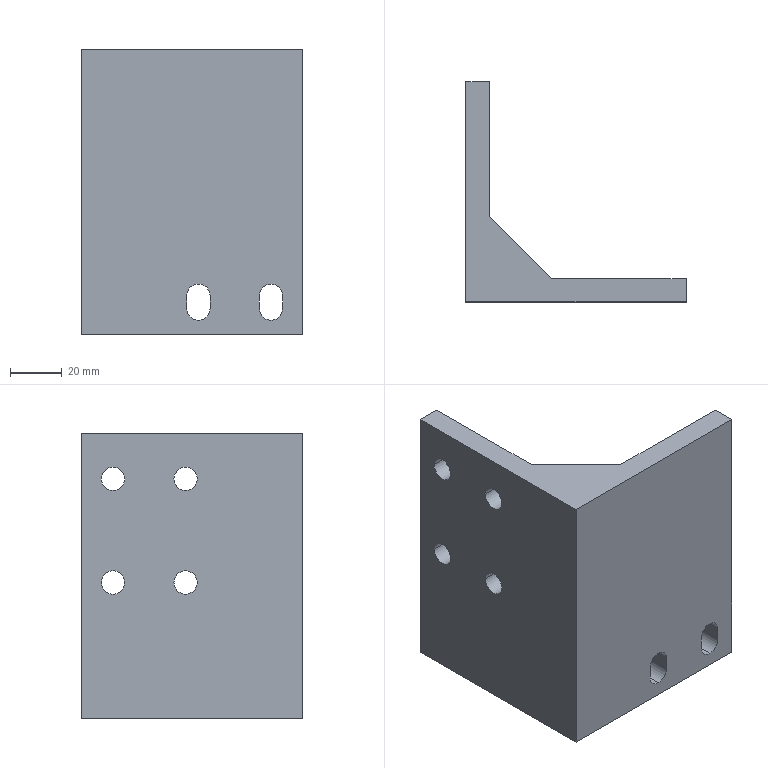Part | 1 solid | 27 faces | box 85 x 85 x 110 mm | volume 186825 mm3 | cylinder 14 | plane 13 | commonest cylinder face diameters 9 x14
STEP:
#1=CARTESIAN_POINT('',(30.5,-33.5,-67.));
#2=VERTEX_POINT('',#1);
#3=CARTESIAN_POINT('',(35.,-33.5,-62.5));
#4=VERTEX_POINT('',#3);
#5=CARTESIAN_POINT('',(30.5,-33.5,-62.5));
#6=DIRECTION('',(0.,-1.,0.));
#7=DIRECTION('',(0.,0.,-1.));
#8=AXIS2_PLACEMENT_3D('',#5,#6,#7);
#9=CIRCLE('',#8,4.5);
#10=EDGE_CURVE('',#2,#4,#9,.T.);
#11=ORIENTED_EDGE('',*,*,#10,.F.);
#12=CARTESIAN_POINT('',(30.5,-42.5,-67.));
#13=VERTEX_POINT('',#12);
#14=CARTESIAN_POINT('',(30.5,42.5,-67.));
#15=DIRECTION('',(0.,-1.,0.));
#16=VECTOR('',#15,1000.);
#17=LINE('',#14,#16);
#18=EDGE_CURVE('',#2,#13,#17,.T.);
#19=ORIENTED_EDGE('',*,*,#18,.T.);
#20=CARTESIAN_POINT('',(35.,-42.5,-62.5));
#21=VERTEX_POINT('',#20);
#22=CARTESIAN_POINT('',(30.5,-42.5,-62.5));
#23=DIRECTION('',(0.,-1.,0.));
#24=DIRECTION('',(0.,0.,-1.));
#25=AXIS2_PLACEMENT_3D('',#22,#23,#24);
#26=CIRCLE('',#25,4.5);
#27=EDGE_CURVE('',#13,#21,#26,.T.);
#28=ORIENTED_EDGE('',*,*,#27,.T.);
#29=CARTESIAN_POINT('',(35.,42.5,-62.5));
#30=DIRECTION('',(0.,-1.,0.));
#31=VECTOR('',#30,1000.);
#32=LINE('',#29,#31);
#33=EDGE_CURVE('',#4,#21,#32,.T.);
#34=ORIENTED_EDGE('',*,*,#33,.F.);
#35=EDGE_LOOP('',(#11,#19,#28,#34));
#36=FACE_OUTER_BOUND('',#35,.T.);
#37=CARTESIAN_POINT('',(30.5,42.5,-62.5));
#38=DIRECTION('',(0.,-1.,0.));
#39=DIRECTION('',(0.,0.,-1.));
#40=AXIS2_PLACEMENT_3D('',#37,#38,#39);
#41=CYLINDRICAL_SURFACE('',#40,4.5);
#42=ADVANCED_FACE('',(#36),#41,.F.);
#43=CARTESIAN_POINT('',(2.5,-33.5,-67.));
#44=VERTEX_POINT('',#43);
#45=CARTESIAN_POINT('',(7.,-33.5,-62.5));
#46=VERTEX_POINT('',#45);
#47=CARTESIAN_POINT('',(2.5,-33.5,-62.5));
#48=DIRECTION('',(0.,-1.,0.));
#49=DIRECTION('',(0.,0.,-1.));
#50=AXIS2_PLACEMENT_3D('',#47,#48,#49);
#51=CIRCLE('',#50,4.5);
#52=EDGE_CURVE('',#44,#46,#51,.T.);
#53=ORIENTED_EDGE('',*,*,#52,.F.);
#54=CARTESIAN_POINT('',(2.5,-42.5,-67.));
#55=VERTEX_POINT('',#54);
#56=CARTESIAN_POINT('',(2.5,42.5,-67.));
#57=DIRECTION('',(0.,-1.,0.));
#58=VECTOR('',#57,1000.);
#59=LINE('',#56,#58);
#60=EDGE_CURVE('',#44,#55,#59,.T.);
#61=ORIENTED_EDGE('',*,*,#60,.T.);
#62=CARTESIAN_POINT('',(7.,-42.5,-62.5));
#63=VERTEX_POINT('',#62);
#64=CARTESIAN_POINT('',(2.5,-42.5,-62.5));
#65=DIRECTION('',(0.,-1.,0.));
#66=DIRECTION('',(0.,0.,-1.));
#67=AXIS2_PLACEMENT_3D('',#64,#65,#66);
#68=CIRCLE('',#67,4.5);
#69=EDGE_CURVE('',#55,#63,#68,.T.);
#70=ORIENTED_EDGE('',*,*,#69,.T.);
#71=CARTESIAN_POINT('',(7.,42.5,-62.5));
#72=DIRECTION('',(0.,-1.,0.));
#73=VECTOR('',#72,1000.);
#74=LINE('',#71,#73);
#75=EDGE_CURVE('',#46,#63,#74,.T.);
#76=ORIENTED_EDGE('',*,*,#75,.F.);
#77=EDGE_LOOP('',(#53,#61,#70,#76));
#78=FACE_OUTER_BOUND('',#77,.T.);
#79=CARTESIAN_POINT('',(2.5,42.5,-62.5));
#80=DIRECTION('',(0.,-1.,0.));
#81=DIRECTION('',(0.,0.,-1.));
#82=AXIS2_PLACEMENT_3D('',#79,#80,#81);
#83=CYLINDRICAL_SURFACE('',#82,4.5);
#84=ADVANCED_FACE('',(#78),#83,.F.);
#85=CARTESIAN_POINT('',(-42.5,-2.,-20.));
#86=VERTEX_POINT('',#85);
#87=CARTESIAN_POINT('',(-42.5,7.,-20.));
#88=VERTEX_POINT('',#87);
#89=CARTESIAN_POINT('',(-42.5,2.5,-20.));
#90=DIRECTION('',(1.,0.,0.));
#91=DIRECTION('',(0.,1.,0.));
#92=AXIS2_PLACEMENT_3D('',#89,#90,#91);
#93=CIRCLE('',#92,4.5);
#94=EDGE_CURVE('',#86,#88,#93,.T.);
#95=ORIENTED_EDGE('',*,*,#94,.F.);
#96=CARTESIAN_POINT('',(-33.5,-2.,-20.));
#97=VERTEX_POINT('',#96);
#98=CARTESIAN_POINT('',(-42.5,-2.,-20.));
#99=DIRECTION('',(1.,0.,0.));
#100=VECTOR('',#99,1000.);
#101=LINE('',#98,#100);
#102=EDGE_CURVE('',#86,#97,#101,.T.);
#103=ORIENTED_EDGE('',*,*,#102,.T.);
#104=CARTESIAN_POINT('',(-33.5,7.,-20.));
#105=VERTEX_POINT('',#104);
#106=CARTESIAN_POINT('',(-33.5,2.5,-20.));
#107=DIRECTION('',(1.,0.,0.));
#108=DIRECTION('',(0.,1.,0.));
#109=AXIS2_PLACEMENT_3D('',#106,#107,#108);
#110=CIRCLE('',#109,4.5);
#111=EDGE_CURVE('',#97,#105,#110,.T.);
#112=ORIENTED_EDGE('',*,*,#111,.T.);
#113=CARTESIAN_POINT('',(-42.5,7.,-20.));
#114=DIRECTION('',(1.,0.,0.));
#115=VECTOR('',#114,1000.);
#116=LINE('',#113,#115);
#117=EDGE_CURVE('',#88,#105,#116,.T.);
#118=ORIENTED_EDGE('',*,*,#117,.F.);
#119=EDGE_LOOP('',(#95,#103,#112,#118));
#120=FACE_OUTER_BOUND('',#119,.T.);
#121=CARTESIAN_POINT('',(-42.5,2.5,-20.));
#122=DIRECTION('',(1.,0.,0.));
#123=DIRECTION('',(0.,1.,0.));
#124=AXIS2_PLACEMENT_3D('',#121,#122,#123);
#125=CYLINDRICAL_SURFACE('',#124,4.5);
#126=ADVANCED_FACE('',(#120),#125,.F.);
#127=CARTESIAN_POINT('',(-42.5,-2.,20.));
#128=VERTEX_POINT('',#127);
#129=CARTESIAN_POINT('',(-42.5,7.,20.));
#130=VERTEX_POINT('',#129);
#131=CARTESIAN_POINT('',(-42.5,2.5,20.));
#132=DIRECTION('',(1.,0.,0.));
#133=DIRECTION('',(0.,1.,0.));
#134=AXIS2_PLACEMENT_3D('',#131,#132,#133);
#135=CIRCLE('',#134,4.5);
#136=EDGE_CURVE('',#128,#130,#135,.T.);
#137=ORIENTED_EDGE('',*,*,#136,.F.);
#138=CARTESIAN_POINT('',(-33.5,-2.,20.));
#139=VERTEX_POINT('',#138);
#140=CARTESIAN_POINT('',(-42.5,-2.,20.));
#141=DIRECTION('',(1.,0.,0.));
#142=VECTOR('',#141,1000.);
#143=LINE('',#140,#142);
#144=EDGE_CURVE('',#128,#139,#143,.T.);
#145=ORIENTED_EDGE('',*,*,#144,.T.);
#146=CARTESIAN_POINT('',(-33.5,7.,20.));
#147=VERTEX_POINT('',#146);
#148=CARTESIAN_POINT('',(-33.5,2.5,20.));
#149=DIRECTION('',(1.,0.,0.));
#150=DIRECTION('',(0.,1.,0.));
#151=AXIS2_PLACEMENT_3D('',#148,#149,#150);
#152=CIRCLE('',#151,4.5);
#153=EDGE_CURVE('',#139,#147,#152,.T.);
#154=ORIENTED_EDGE('',*,*,#153,.T.);
#155=CARTESIAN_POINT('',(-42.5,7.,20.));
#156=DIRECTION('',(1.,0.,0.));
#157=VECTOR('',#156,1000.);
#158=LINE('',#155,#157);
#159=EDGE_CURVE('',#130,#147,#158,.T.);
#160=ORIENTED_EDGE('',*,*,#159,.F.);
#161=EDGE_LOOP('',(#137,#145,#154,#160));
#162=FACE_OUTER_BOUND('',#161,.T.);
#163=CARTESIAN_POINT('',(-42.5,2.5,20.));
#164=DIRECTION('',(1.,0.,0.));
#165=DIRECTION('',(0.,1.,0.));
#166=AXIS2_PLACEMENT_3D('',#163,#164,#165);
#167=CYLINDRICAL_SURFACE('',#166,4.5);
#168=ADVANCED_FACE('',(#162),#167,.F.);
#169=CARTESIAN_POINT('',(-42.5,26.,20.));
#170=VERTEX_POINT('',#169);
#171=CARTESIAN_POINT('',(-42.5,35.,20.));
#172=VERTEX_POINT('',#171);
#173=CARTESIAN_POINT('',(-42.5,30.5,20.));
#174=DIRECTION('',(1.,0.,0.));
#175=DIRECTION('',(0.,1.,0.));
#176=AXIS2_PLACEMENT_3D('',#173,#174,#175);
#177=CIRCLE('',#176,4.5);
#178=EDGE_CURVE('',#170,#172,#177,.T.);
#179=ORIENTED_EDGE('',*,*,#178,.F.);
#180=CARTESIAN_POINT('',(-33.5,26.,20.));
#181=VERTEX_POINT('',#180);
#182=CARTESIAN_POINT('',(-42.5,26.,20.));
#183=DIRECTION('',(1.,0.,0.));
#184=VECTOR('',#183,1000.);
#185=LINE('',#182,#184);
#186=EDGE_CURVE('',#170,#181,#185,.T.);
#187=ORIENTED_EDGE('',*,*,#186,.T.);
#188=CARTESIAN_POINT('',(-33.5,35.,20.));
#189=VERTEX_POINT('',#188);
#190=CARTESIAN_POINT('',(-33.5,30.5,20.));
#191=DIRECTION('',(1.,0.,0.));
#192=DIRECTION('',(0.,1.,0.));
#193=AXIS2_PLACEMENT_3D('',#190,#191,#192);
#194=CIRCLE('',#193,4.5);
#195=EDGE_CURVE('',#181,#189,#194,.T.);
#196=ORIENTED_EDGE('',*,*,#195,.T.);
#197=CARTESIAN_POINT('',(-42.5,35.,20.));
#198=DIRECTION('',(1.,0.,0.));
#199=VECTOR('',#198,1000.);
#200=LINE('',#197,#199);
#201=EDGE_CURVE('',#172,#189,#200,.T.);
#202=ORIENTED_EDGE('',*,*,#201,.F.);
#203=EDGE_LOOP('',(#179,#187,#196,#202));
#204=FACE_OUTER_BOUND('',#203,.T.);
#205=CARTESIAN_POINT('',(-42.5,30.5,20.));
#206=DIRECTION('',(1.,0.,0.));
#207=DIRECTION('',(0.,1.,0.));
#208=AXIS2_PLACEMENT_3D('',#205,#206,#207);
#209=CYLINDRICAL_SURFACE('',#208,4.5);
#210=ADVANCED_FACE('',(#204),#209,.F.);
#211=CARTESIAN_POINT('',(-42.5,26.,-20.));
#212=VERTEX_POINT('',#211);
#213=CARTESIAN_POINT('',(-42.5,35.,-20.));
#214=VERTEX_POINT('',#213);
#215=CARTESIAN_POINT('',(-42.5,30.5,-20.));
#216=DIRECTION('',(1.,0.,0.));
#217=DIRECTION('',(0.,1.,0.));
#218=AXIS2_PLACEMENT_3D('',#215,#216,#217);
#219=CIRCLE('',#218,4.5);
#220=EDGE_CURVE('',#212,#214,#219,.T.);
#221=ORIENTED_EDGE('',*,*,#220,.F.);
#222=CARTESIAN_POINT('',(-33.5,26.,-20.));
#223=VERTEX_POINT('',#222);
#224=CARTESIAN_POINT('',(-42.5,26.,-20.));
#225=DIRECTION('',(1.,0.,0.));
#226=VECTOR('',#225,1000.);
#227=LINE('',#224,#226);
#228=EDGE_CURVE('',#212,#223,#227,.T.);
#229=ORIENTED_EDGE('',*,*,#228,.T.);
#230=CARTESIAN_POINT('',(-33.5,35.,-20.));
#231=VERTEX_POINT('',#230);
#232=CARTESIAN_POINT('',(-33.5,30.5,-20.));
#233=DIRECTION('',(1.,0.,0.));
#234=DIRECTION('',(0.,1.,0.));
#235=AXIS2_PLACEMENT_3D('',#232,#233,#234);
#236=CIRCLE('',#235,4.5);
#237=EDGE_CURVE('',#223,#231,#236,.T.);
#238=ORIENTED_EDGE('',*,*,#237,.T.);
#239=CARTESIAN_POINT('',(-42.5,35.,-20.));
#240=DIRECTION('',(1.,0.,0.));
#241=VECTOR('',#240,1000.);
#242=LINE('',#239,#241);
#243=EDGE_CURVE('',#214,#231,#242,.T.);
#244=ORIENTED_EDGE('',*,*,#243,.F.);
#245=EDGE_LOOP('',(#221,#229,#238,#244));
#246=FACE_OUTER_BOUND('',#245,.T.);
#247=CARTESIAN_POINT('',(-42.5,30.5,-20.));
#248=DIRECTION('',(1.,0.,0.));
#249=DIRECTION('',(0.,1.,0.));
#250=AXIS2_PLACEMENT_3D('',#247,#248,#249);
#251=CYLINDRICAL_SURFACE('',#250,4.5);
#252=ADVANCED_FACE('',(#246),#251,.F.);
#253=CARTESIAN_POINT('',(-33.5,42.5,37.5));
#254=VERTEX_POINT('',#253);
#255=CARTESIAN_POINT('',(-33.5,42.5,-72.5));
#256=VERTEX_POINT('',#255);
#257=CARTESIAN_POINT('',(-33.5,42.5,37.5));
#258=DIRECTION('',(0.,0.,-1.));
#259=VECTOR('',#258,1000.);
#260=LINE('',#257,#259);
#261=EDGE_CURVE('',#254,#256,#260,.T.);
#262=ORIENTED_EDGE('',*,*,#261,.T.);
#263=CARTESIAN_POINT('',(-42.5,42.5,-72.5));
#264=VERTEX_POINT('',#263);
#265=CARTESIAN_POINT('',(42.5,42.5,-72.5));
#266=DIRECTION('',(-1.,0.,0.));
#267=VECTOR('',#266,1000.);
#268=LINE('',#265,#267);
#269=EDGE_CURVE('',#256,#264,#268,.T.);
#270=ORIENTED_EDGE('',*,*,#269,.T.);
#271=CARTESIAN_POINT('',(-42.5,42.5,37.5));
#272=VERTEX_POINT('',#271);
#273=CARTESIAN_POINT('',(-42.5,42.5,-37.5));
#274=DIRECTION('',(0.,0.,1.));
#275=VECTOR('',#274,1000.);
#276=LINE('',#273,#275);
#277=EDGE_CURVE('',#264,#272,#276,.T.);
#278=ORIENTED_EDGE('',*,*,#277,.T.);
#279=CARTESIAN_POINT('',(42.5,42.5,37.5));
#280=DIRECTION('',(-1.,0.,0.));
#281=VECTOR('',#280,1000.);
#282=LINE('',#279,#281);
#283=EDGE_CURVE('',#254,#272,#282,.T.);
#284=ORIENTED_EDGE('',*,*,#283,.F.);
#285=EDGE_LOOP('',(#262,#270,#278,#284));
#286=FACE_OUTER_BOUND('',#285,.T.);
#287=CARTESIAN_POINT('',(42.5,42.5,-37.5));
#288=DIRECTION('',(0.,1.,0.));
#289=DIRECTION('',(-1.,0.,0.));
#290=AXIS2_PLACEMENT_3D('',#287,#288,#289);
#291=PLANE('',#290);
#292=ADVANCED_FACE('',(#286),#291,.T.);
#293=CARTESIAN_POINT('',(42.5,-33.5,37.5));
#294=VERTEX_POINT('',#293);
#295=CARTESIAN_POINT('',(42.5,-33.5,-72.5));
#296=VERTEX_POINT('',#295);
#297=CARTESIAN_POINT('',(42.5,-33.5,37.5));
#298=DIRECTION('',(0.,0.,-1.));
#299=VECTOR('',#298,1000.);
#300=LINE('',#297,#299);
#301=EDGE_CURVE('',#294,#296,#300,.T.);
#302=ORIENTED_EDGE('',*,*,#301,.F.);
#303=CARTESIAN_POINT('',(42.5,-42.5,37.5));
#304=VERTEX_POINT('',#303);
#305=CARTESIAN_POINT('',(42.5,-42.5,37.5));
#306=DIRECTION('',(0.,1.,0.));
#307=VECTOR('',#306,1000.);
#308=LINE('',#305,#307);
#309=EDGE_CURVE('',#304,#294,#308,.T.);
#310=ORIENTED_EDGE('',*,*,#309,.F.);
#311=CARTESIAN_POINT('',(42.5,-42.5,-72.5));
#312=VERTEX_POINT('',#311);
#313=CARTESIAN_POINT('',(42.5,-42.5,-37.5));
#314=DIRECTION('',(0.,0.,1.));
#315=VECTOR('',#314,1000.);
#316=LINE('',#313,#315);
#317=EDGE_CURVE('',#312,#304,#316,.T.);
#318=ORIENTED_EDGE('',*,*,#317,.F.);
#319=CARTESIAN_POINT('',(42.5,-42.5,-72.5));
#320=DIRECTION('',(0.,1.,0.));
#321=VECTOR('',#320,1000.);
#322=LINE('',#319,#321);
#323=EDGE_CURVE('',#312,#296,#322,.T.);
#324=ORIENTED_EDGE('',*,*,#323,.T.);
#325=EDGE_LOOP('',(#302,#310,#318,#324));
#326=FACE_OUTER_BOUND('',#325,.T.);
#327=CARTESIAN_POINT('',(42.5,-42.5,-37.5));
#328=DIRECTION('',(1.,0.,0.));
#329=DIRECTION('',(0.,0.,-1.));
#330=AXIS2_PLACEMENT_3D('',#327,#328,#329);
#331=PLANE('',#330);
#332=ADVANCED_FACE('',(#326),#331,.T.);
#333=CARTESIAN_POINT('',(26.,-42.5,-62.5));
#334=VERTEX_POINT('',#333);
#335=CARTESIAN_POINT('',(30.5,-42.5,-62.5));
#336=DIRECTION('',(0.,-1.,0.));
#337=DIRECTION('',(0.,0.,-1.));
#338=AXIS2_PLACEMENT_3D('',#335,#336,#337);
#339=CIRCLE('',#338,4.5);
#340=EDGE_CURVE('',#334,#13,#339,.T.);
#341=ORIENTED_EDGE('',*,*,#340,.F.);
#342=CARTESIAN_POINT('',(26.,-42.5,-57.5));
#343=VERTEX_POINT('',#342);
#344=CARTESIAN_POINT('',(26.,-42.5,-62.5));
#345=DIRECTION('',(0.,0.,-1.));
#346=VECTOR('',#345,1000.);
#347=LINE('',#344,#346);
#348=EDGE_CURVE('',#343,#334,#347,.T.);
#349=ORIENTED_EDGE('',*,*,#348,.F.);
#350=CARTESIAN_POINT('',(35.,-42.5,-57.5));
#351=VERTEX_POINT('',#350);
#352=CARTESIAN_POINT('',(30.5,-42.5,-57.5));
#353=DIRECTION('',(0.,-1.,0.));
#354=DIRECTION('',(0.,0.,-1.));
#355=AXIS2_PLACEMENT_3D('',#352,#353,#354);
#356=CIRCLE('',#355,4.5);
#357=EDGE_CURVE('',#351,#343,#356,.T.);
#358=ORIENTED_EDGE('',*,*,#357,.F.);
#359=CARTESIAN_POINT('',(35.,-42.5,-62.5));
#360=DIRECTION('',(0.,0.,1.));
#361=VECTOR('',#360,1000.);
#362=LINE('',#359,#361);
#363=EDGE_CURVE('',#21,#351,#362,.T.);
#364=ORIENTED_EDGE('',*,*,#363,.F.);
#365=ORIENTED_EDGE('',*,*,#27,.F.);
#366=EDGE_LOOP('',(#341,#349,#358,#364,#365));
#367=FACE_BOUND('',#366,.T.);
#368=CARTESIAN_POINT('',(-2.,-42.5,-62.5));
#369=VERTEX_POINT('',#368);
#370=CARTESIAN_POINT('',(2.5,-42.5,-62.5));
#371=DIRECTION('',(0.,-1.,0.));
#372=DIRECTION('',(0.,0.,-1.));
#373=AXIS2_PLACEMENT_3D('',#370,#371,#372);
#374=CIRCLE('',#373,4.5);
#375=EDGE_CURVE('',#369,#55,#374,.T.);
#376=ORIENTED_EDGE('',*,*,#375,.F.);
#377=CARTESIAN_POINT('',(-2.,-42.5,-57.5));
#378=VERTEX_POINT('',#377);
#379=CARTESIAN_POINT('',(-2.,-42.5,-62.5));
#380=DIRECTION('',(0.,0.,-1.));
#381=VECTOR('',#380,1000.);
#382=LINE('',#379,#381);
#383=EDGE_CURVE('',#378,#369,#382,.T.);
#384=ORIENTED_EDGE('',*,*,#383,.F.);
#385=CARTESIAN_POINT('',(7.,-42.5,-57.5));
#386=VERTEX_POINT('',#385);
#387=CARTESIAN_POINT('',(2.5,-42.5,-57.5));
#388=DIRECTION('',(0.,-1.,0.));
#389=DIRECTION('',(0.,0.,-1.));
#390=AXIS2_PLACEMENT_3D('',#387,#388,#389);
#391=CIRCLE('',#390,4.5);
#392=EDGE_CURVE('',#386,#378,#391,.T.);
#393=ORIENTED_EDGE('',*,*,#392,.F.);
#394=CARTESIAN_POINT('',(7.,-42.5,-62.5));
#395=DIRECTION('',(0.,0.,1.));
#396=VECTOR('',#395,1000.);
#397=LINE('',#394,#396);
#398=EDGE_CURVE('',#63,#386,#397,.T.);
#399=ORIENTED_EDGE('',*,*,#398,.F.);
#400=ORIENTED_EDGE('',*,*,#69,.F.);
#401=EDGE_LOOP('',(#376,#384,#393,#399,#400));
#402=FACE_BOUND('',#401,.T.);
#403=CARTESIAN_POINT('',(-42.5,-42.5,37.5));
#404=VERTEX_POINT('',#403);
#405=CARTESIAN_POINT('',(-42.5,-42.5,37.5));
#406=DIRECTION('',(1.,0.,0.));
#407=VECTOR('',#406,1000.);
#408=LINE('',#405,#407);
#409=EDGE_CURVE('',#404,#304,#408,.T.);
#410=ORIENTED_EDGE('',*,*,#409,.F.);
#411=CARTESIAN_POINT('',(-42.5,-42.5,-72.5));
#412=VERTEX_POINT('',#411);
#413=CARTESIAN_POINT('',(-42.5,-42.5,-37.5));
#414=DIRECTION('',(0.,0.,1.));
#415=VECTOR('',#414,1000.);
#416=LINE('',#413,#415);
#417=EDGE_CURVE('',#412,#404,#416,.T.);
#418=ORIENTED_EDGE('',*,*,#417,.F.);
#419=CARTESIAN_POINT('',(-42.5,-42.5,-72.5));
#420=DIRECTION('',(1.,0.,0.));
#421=VECTOR('',#420,1000.);
#422=LINE('',#419,#421);
#423=EDGE_CURVE('',#412,#312,#422,.T.);
#424=ORIENTED_EDGE('',*,*,#423,.T.);
#425=ORIENTED_EDGE('',*,*,#317,.T.);
#426=EDGE_LOOP('',(#410,#418,#424,#425));
#427=FACE_OUTER_BOUND('',#426,.T.);
#428=CARTESIAN_POINT('',(-42.5,-42.5,-37.5));
#429=DIRECTION('',(0.,-1.,0.));
#430=DIRECTION('',(0.,0.,-1.));
#431=AXIS2_PLACEMENT_3D('',#428,#429,#430);
#432=PLANE('',#431);
#433=ADVANCED_FACE('',(#367,#402,#427),#432,.T.);
#434=CARTESIAN_POINT('',(-42.5,2.5,-20.));
#435=DIRECTION('',(1.,0.,0.));
#436=DIRECTION('',(0.,1.,0.));
#437=AXIS2_PLACEMENT_3D('',#434,#435,#436);
#438=CIRCLE('',#437,4.5);
#439=EDGE_CURVE('',#88,#86,#438,.T.);
#440=ORIENTED_EDGE('',*,*,#439,.T.);
#441=ORIENTED_EDGE('',*,*,#94,.T.);
#442=EDGE_LOOP('',(#440,#441));
#443=FACE_BOUND('',#442,.T.);
#444=CARTESIAN_POINT('',(-42.5,2.5,20.));
#445=DIRECTION('',(1.,0.,0.));
#446=DIRECTION('',(0.,1.,0.));
#447=AXIS2_PLACEMENT_3D('',#444,#445,#446);
#448=CIRCLE('',#447,4.5);
#449=EDGE_CURVE('',#130,#128,#448,.T.);
#450=ORIENTED_EDGE('',*,*,#449,.T.);
#451=ORIENTED_EDGE('',*,*,#136,.T.);
#452=EDGE_LOOP('',(#450,#451));
#453=FACE_BOUND('',#452,.T.);
#454=CARTESIAN_POINT('',(-42.5,30.5,20.));
#455=DIRECTION('',(1.,0.,0.));
#456=DIRECTION('',(0.,1.,0.));
#457=AXIS2_PLACEMENT_3D('',#454,#455,#456);
#458=CIRCLE('',#457,4.5);
#459=EDGE_CURVE('',#172,#170,#458,.T.);
#460=ORIENTED_EDGE('',*,*,#459,.T.);
#461=ORIENTED_EDGE('',*,*,#178,.T.);
#462=EDGE_LOOP('',(#460,#461));
#463=FACE_BOUND('',#462,.T.);
#464=CARTESIAN_POINT('',(-42.5,30.5,-20.));
#465=DIRECTION('',(1.,0.,0.));
#466=DIRECTION('',(0.,1.,0.));
#467=AXIS2_PLACEMENT_3D('',#464,#465,#466);
#468=CIRCLE('',#467,4.5);
#469=EDGE_CURVE('',#214,#212,#468,.T.);
#470=ORIENTED_EDGE('',*,*,#469,.T.);
#471=ORIENTED_EDGE('',*,*,#220,.T.);
#472=EDGE_LOOP('',(#470,#471));
#473=FACE_BOUND('',#472,.T.);
#474=CARTESIAN_POINT('',(-42.5,42.5,37.5));
#475=DIRECTION('',(0.,-1.,0.));
#476=VECTOR('',#475,1000.);
#477=LINE('',#474,#476);
#478=EDGE_CURVE('',#272,#404,#477,.T.);
#479=ORIENTED_EDGE('',*,*,#478,.F.);
#480=ORIENTED_EDGE('',*,*,#277,.F.);
#481=CARTESIAN_POINT('',(-42.5,42.5,-72.5));
#482=DIRECTION('',(0.,-1.,0.));
#483=VECTOR('',#482,1000.);
#484=LINE('',#481,#483);
#485=EDGE_CURVE('',#264,#412,#484,.T.);
#486=ORIENTED_EDGE('',*,*,#485,.T.);
#487=ORIENTED_EDGE('',*,*,#417,.T.);
#488=EDGE_LOOP('',(#479,#480,#486,#487));
#489=FACE_OUTER_BOUND('',#488,.T.);
#490=CARTESIAN_POINT('',(-42.5,42.5,-37.5));
#491=DIRECTION('',(-1.,0.,0.));
#492=DIRECTION('',(0.,-1.,0.));
#493=AXIS2_PLACEMENT_3D('',#490,#491,#492);
#494=PLANE('',#493);
#495=ADVANCED_FACE('',(#443,#453,#463,#473,#489),#494,.T.);
#496=ORIENTED_EDGE('',*,*,#269,.F.);
#497=CARTESIAN_POINT('',(-33.5,-9.5,-72.5));
#498=VERTEX_POINT('',#497);
#499=CARTESIAN_POINT('',(-33.5,-33.5,-72.5));
#500=DIRECTION('',(0.,1.,0.));
#501=VECTOR('',#500,1000.);
#502=LINE('',#499,#501);
#503=EDGE_CURVE('',#498,#256,#502,.T.);
#504=ORIENTED_EDGE('',*,*,#503,.F.);
#505=CARTESIAN_POINT('',(-9.5,-33.5,-72.5));
#506=VERTEX_POINT('',#505);
#507=CARTESIAN_POINT('',(-21.5,-21.5,-72.5));
#508=DIRECTION('',(0.7071,-0.7071,0.));
#509=VECTOR('',#508,1000.);
#510=LINE('',#507,#509);
#511=EDGE_CURVE('',#498,#506,#510,.T.);
#512=ORIENTED_EDGE('',*,*,#511,.T.);
#513=CARTESIAN_POINT('',(42.5,-33.5,-72.5));
#514=DIRECTION('',(-1.,0.,0.));
#515=VECTOR('',#514,1000.);
#516=LINE('',#513,#515);
#517=EDGE_CURVE('',#296,#506,#516,.T.);
#518=ORIENTED_EDGE('',*,*,#517,.F.);
#519=ORIENTED_EDGE('',*,*,#323,.F.);
#520=ORIENTED_EDGE('',*,*,#423,.F.);
#521=ORIENTED_EDGE('',*,*,#485,.F.);
#522=EDGE_LOOP('',(#496,#504,#512,#518,#519,#520,#521));
#523=FACE_OUTER_BOUND('',#522,.T.);
#524=CARTESIAN_POINT('',(0.,0.,-72.5));
#525=DIRECTION('',(0.,0.,1.));
#526=DIRECTION('',(1.,0.,0.));
#527=AXIS2_PLACEMENT_3D('',#524,#525,#526);
#528=PLANE('',#527);
#529=ADVANCED_FACE('',(#523),#528,.F.);
#530=CARTESIAN_POINT('',(-9.5,-33.5,37.5));
#531=VERTEX_POINT('',#530);
#532=CARTESIAN_POINT('',(42.5,-33.5,37.5));
#533=DIRECTION('',(-1.,0.,0.));
#534=VECTOR('',#533,1000.);
#535=LINE('',#532,#534);
#536=EDGE_CURVE('',#294,#531,#535,.T.);
#537=ORIENTED_EDGE('',*,*,#536,.T.);
#538=CARTESIAN_POINT('',(-33.5,-9.5,37.5));
#539=VERTEX_POINT('',#538);
#540=CARTESIAN_POINT('',(-33.5,-9.5,37.5));
#541=DIRECTION('',(-0.7071,0.7071,0.));
#542=VECTOR('',#541,1000.);
#543=LINE('',#540,#542);
#544=EDGE_CURVE('',#531,#539,#543,.T.);
#545=ORIENTED_EDGE('',*,*,#544,.T.);
#546=CARTESIAN_POINT('',(-33.5,-33.5,37.5));
#547=DIRECTION('',(0.,1.,0.));
#548=VECTOR('',#547,1000.);
#549=LINE('',#546,#548);
#550=EDGE_CURVE('',#539,#254,#549,.T.);
#551=ORIENTED_EDGE('',*,*,#550,.T.);
#552=ORIENTED_EDGE('',*,*,#283,.T.);
#553=ORIENTED_EDGE('',*,*,#478,.T.);
#554=ORIENTED_EDGE('',*,*,#409,.T.);
#555=ORIENTED_EDGE('',*,*,#309,.T.);
#556=EDGE_LOOP('',(#537,#545,#551,#552,#553,#554,#555));
#557=FACE_OUTER_BOUND('',#556,.T.);
#558=CARTESIAN_POINT('',(0.,0.,37.5));
#559=DIRECTION('',(0.,0.,1.));
#560=DIRECTION('',(1.,0.,0.));
#561=AXIS2_PLACEMENT_3D('',#558,#559,#560);
#562=PLANE('',#561);
#563=ADVANCED_FACE('',(#557),#562,.T.);
#564=CARTESIAN_POINT('',(-33.5,2.5,-20.));
#565=DIRECTION('',(1.,0.,0.));
#566=DIRECTION('',(0.,1.,0.));
#567=AXIS2_PLACEMENT_3D('',#564,#565,#566);
#568=CIRCLE('',#567,4.5);
#569=EDGE_CURVE('',#105,#97,#568,.T.);
#570=ORIENTED_EDGE('',*,*,#569,.F.);
#571=ORIENTED_EDGE('',*,*,#111,.F.);
#572=EDGE_LOOP('',(#570,#571));
#573=FACE_BOUND('',#572,.T.);
#574=CARTESIAN_POINT('',(-33.5,2.5,20.));
#575=DIRECTION('',(1.,0.,0.));
#576=DIRECTION('',(0.,1.,0.));
#577=AXIS2_PLACEMENT_3D('',#574,#575,#576);
#578=CIRCLE('',#577,4.5);
#579=EDGE_CURVE('',#147,#139,#578,.T.);
#580=ORIENTED_EDGE('',*,*,#579,.F.);
#581=ORIENTED_EDGE('',*,*,#153,.F.);
#582=EDGE_LOOP('',(#580,#581));
#583=FACE_BOUND('',#582,.T.);
#584=CARTESIAN_POINT('',(-33.5,30.5,20.));
#585=DIRECTION('',(1.,0.,0.));
#586=DIRECTION('',(0.,1.,0.));
#587=AXIS2_PLACEMENT_3D('',#584,#585,#586);
#588=CIRCLE('',#587,4.5);
#589=EDGE_CURVE('',#189,#181,#588,.T.);
#590=ORIENTED_EDGE('',*,*,#589,.F.);
#591=ORIENTED_EDGE('',*,*,#195,.F.);
#592=EDGE_LOOP('',(#590,#591));
#593=FACE_BOUND('',#592,.T.);
#594=CARTESIAN_POINT('',(-33.5,30.5,-20.));
#595=DIRECTION('',(1.,0.,0.));
#596=DIRECTION('',(0.,1.,0.));
#597=AXIS2_PLACEMENT_3D('',#594,#595,#596);
#598=CIRCLE('',#597,4.5);
#599=EDGE_CURVE('',#231,#223,#598,.T.);
#600=ORIENTED_EDGE('',*,*,#599,.F.);
#601=ORIENTED_EDGE('',*,*,#237,.F.);
#602=EDGE_LOOP('',(#600,#601));
#603=FACE_BOUND('',#602,.T.);
#604=ORIENTED_EDGE('',*,*,#550,.F.);
#605=CARTESIAN_POINT('',(-33.5,-9.5,-37.5));
#606=DIRECTION('',(0.,0.,-1.));
#607=VECTOR('',#606,1000.);
#608=LINE('',#605,#607);
#609=EDGE_CURVE('',#539,#498,#608,.T.);
#610=ORIENTED_EDGE('',*,*,#609,.T.);
#611=ORIENTED_EDGE('',*,*,#503,.T.);
#612=ORIENTED_EDGE('',*,*,#261,.F.);
#613=EDGE_LOOP('',(#604,#610,#611,#612));
#614=FACE_OUTER_BOUND('',#613,.T.);
#615=CARTESIAN_POINT('',(-33.5,-33.5,37.5));
#616=DIRECTION('',(-1.,0.,0.));
#617=DIRECTION('',(0.,-1.,0.));
#618=AXIS2_PLACEMENT_3D('',#615,#616,#617);
#619=PLANE('',#618);
#620=ADVANCED_FACE('',(#573,#583,#593,#603,#614),#619,.F.);
#621=CARTESIAN_POINT('',(26.,-33.5,-57.5));
#622=VERTEX_POINT('',#621);
#623=CARTESIAN_POINT('',(26.,-33.5,-62.5));
#624=VERTEX_POINT('',#623);
#625=CARTESIAN_POINT('',(26.,-33.5,37.5));
#626=DIRECTION('',(0.,0.,-1.));
#627=VECTOR('',#626,1000.);
#628=LINE('',#625,#627);
#629=EDGE_CURVE('',#622,#624,#628,.T.);
#630=ORIENTED_EDGE('',*,*,#629,.T.);
#631=CARTESIAN_POINT('',(30.5,-33.5,-62.5));
#632=DIRECTION('',(0.,-1.,0.));
#633=DIRECTION('',(0.,0.,-1.));
#634=AXIS2_PLACEMENT_3D('',#631,#632,#633);
#635=CIRCLE('',#634,4.5);
#636=EDGE_CURVE('',#624,#2,#635,.T.);
#637=ORIENTED_EDGE('',*,*,#636,.T.);
#638=ORIENTED_EDGE('',*,*,#10,.T.);
#639=CARTESIAN_POINT('',(35.,-33.5,-57.5));
#640=VERTEX_POINT('',#639);
#641=CARTESIAN_POINT('',(35.,-33.5,37.5));
#642=DIRECTION('',(0.,0.,1.));
#643=VECTOR('',#642,1000.);
#644=LINE('',#641,#643);
#645=EDGE_CURVE('',#4,#640,#644,.T.);
#646=ORIENTED_EDGE('',*,*,#645,.T.);
#647=CARTESIAN_POINT('',(30.5,-33.5,-57.5));
#648=DIRECTION('',(0.,-1.,0.));
#649=DIRECTION('',(0.,0.,-1.));
#650=AXIS2_PLACEMENT_3D('',#647,#648,#649);
#651=CIRCLE('',#650,4.5);
#652=EDGE_CURVE('',#640,#622,#651,.T.);
#653=ORIENTED_EDGE('',*,*,#652,.T.);
#654=EDGE_LOOP('',(#630,#637,#638,#646,#653));
#655=FACE_BOUND('',#654,.T.);
#656=CARTESIAN_POINT('',(-2.,-33.5,-57.5));
#657=VERTEX_POINT('',#656);
#658=CARTESIAN_POINT('',(-2.,-33.5,-62.5));
#659=VERTEX_POINT('',#658);
#660=CARTESIAN_POINT('',(-2.,-33.5,37.5));
#661=DIRECTION('',(0.,0.,-1.));
#662=VECTOR('',#661,1000.);
#663=LINE('',#660,#662);
#664=EDGE_CURVE('',#657,#659,#663,.T.);
#665=ORIENTED_EDGE('',*,*,#664,.T.);
#666=CARTESIAN_POINT('',(2.5,-33.5,-62.5));
#667=DIRECTION('',(0.,-1.,0.));
#668=DIRECTION('',(0.,0.,-1.));
#669=AXIS2_PLACEMENT_3D('',#666,#667,#668);
#670=CIRCLE('',#669,4.5);
#671=EDGE_CURVE('',#659,#44,#670,.T.);
#672=ORIENTED_EDGE('',*,*,#671,.T.);
#673=ORIENTED_EDGE('',*,*,#52,.T.);
#674=CARTESIAN_POINT('',(7.,-33.5,-57.5));
#675=VERTEX_POINT('',#674);
#676=CARTESIAN_POINT('',(7.,-33.5,37.5));
#677=DIRECTION('',(0.,0.,1.));
#678=VECTOR('',#677,1000.);
#679=LINE('',#676,#678);
#680=EDGE_CURVE('',#46,#675,#679,.T.);
#681=ORIENTED_EDGE('',*,*,#680,.T.);
#682=CARTESIAN_POINT('',(2.5,-33.5,-57.5));
#683=DIRECTION('',(0.,-1.,0.));
#684=DIRECTION('',(0.,0.,-1.));
#685=AXIS2_PLACEMENT_3D('',#682,#683,#684);
#686=CIRCLE('',#685,4.5);
#687=EDGE_CURVE('',#675,#657,#686,.T.);
#688=ORIENTED_EDGE('',*,*,#687,.T.);
#689=EDGE_LOOP('',(#665,#672,#673,#681,#688));
#690=FACE_BOUND('',#689,.T.);
#691=ORIENTED_EDGE('',*,*,#517,.T.);
#692=CARTESIAN_POINT('',(-9.5,-33.5,37.5));
#693=DIRECTION('',(0.,0.,1.));
#694=VECTOR('',#693,1000.);
#695=LINE('',#692,#694);
#696=EDGE_CURVE('',#506,#531,#695,.T.);
#697=ORIENTED_EDGE('',*,*,#696,.T.);
#698=ORIENTED_EDGE('',*,*,#536,.F.);
#699=ORIENTED_EDGE('',*,*,#301,.T.);
#700=EDGE_LOOP('',(#691,#697,#698,#699));
#701=FACE_OUTER_BOUND('',#700,.T.);
#702=CARTESIAN_POINT('',(42.5,-33.5,37.5));
#703=DIRECTION('',(0.,-1.,0.));
#704=DIRECTION('',(0.,0.,-1.));
#705=AXIS2_PLACEMENT_3D('',#702,#703,#704);
#706=PLANE('',#705);
#707=ADVANCED_FACE('',(#655,#690,#701),#706,.F.);
#708=ORIENTED_EDGE('',*,*,#544,.F.);
#709=ORIENTED_EDGE('',*,*,#696,.F.);
#710=ORIENTED_EDGE('',*,*,#511,.F.);
#711=ORIENTED_EDGE('',*,*,#609,.F.);
#712=EDGE_LOOP('',(#708,#709,#710,#711));
#713=FACE_OUTER_BOUND('',#712,.T.);
#714=CARTESIAN_POINT('',(-33.5,-9.5,37.5));
#715=DIRECTION('',(0.7071,0.7071,0.));
#716=DIRECTION('',(0.,0.,1.));
#717=AXIS2_PLACEMENT_3D('',#714,#715,#716);
#718=PLANE('',#717);
#719=ADVANCED_FACE('',(#713),#718,.T.);
#720=ORIENTED_EDGE('',*,*,#228,.F.);
#721=ORIENTED_EDGE('',*,*,#469,.F.);
#722=ORIENTED_EDGE('',*,*,#243,.T.);
#723=ORIENTED_EDGE('',*,*,#599,.T.);
#724=EDGE_LOOP('',(#720,#721,#722,#723));
#725=FACE_OUTER_BOUND('',#724,.T.);
#726=CARTESIAN_POINT('',(-42.5,30.5,-20.));
#727=DIRECTION('',(1.,0.,0.));
#728=DIRECTION('',(0.,1.,0.));
#729=AXIS2_PLACEMENT_3D('',#726,#727,#728);
#730=CYLINDRICAL_SURFACE('',#729,4.5);
#731=ADVANCED_FACE('',(#725),#730,.F.);
#732=ORIENTED_EDGE('',*,*,#186,.F.);
#733=ORIENTED_EDGE('',*,*,#459,.F.);
#734=ORIENTED_EDGE('',*,*,#201,.T.);
#735=ORIENTED_EDGE('',*,*,#589,.T.);
#736=EDGE_LOOP('',(#732,#733,#734,#735));
#737=FACE_OUTER_BOUND('',#736,.T.);
#738=CARTESIAN_POINT('',(-42.5,30.5,20.));
#739=DIRECTION('',(1.,0.,0.));
#740=DIRECTION('',(0.,1.,0.));
#741=AXIS2_PLACEMENT_3D('',#738,#739,#740);
#742=CYLINDRICAL_SURFACE('',#741,4.5);
#743=ADVANCED_FACE('',(#737),#742,.F.);
#744=ORIENTED_EDGE('',*,*,#144,.F.);
#745=ORIENTED_EDGE('',*,*,#449,.F.);
#746=ORIENTED_EDGE('',*,*,#159,.T.);
#747=ORIENTED_EDGE('',*,*,#579,.T.);
#748=EDGE_LOOP('',(#744,#745,#746,#747));
#749=FACE_OUTER_BOUND('',#748,.T.);
#750=CARTESIAN_POINT('',(-42.5,2.5,20.));
#751=DIRECTION('',(1.,0.,0.));
#752=DIRECTION('',(0.,1.,0.));
#753=AXIS2_PLACEMENT_3D('',#750,#751,#752);
#754=CYLINDRICAL_SURFACE('',#753,4.5);
#755=ADVANCED_FACE('',(#749),#754,.F.);
#756=ORIENTED_EDGE('',*,*,#102,.F.);
#757=ORIENTED_EDGE('',*,*,#439,.F.);
#758=ORIENTED_EDGE('',*,*,#117,.T.);
#759=ORIENTED_EDGE('',*,*,#569,.T.);
#760=EDGE_LOOP('',(#756,#757,#758,#759));
#761=FACE_OUTER_BOUND('',#760,.T.);
#762=CARTESIAN_POINT('',(-42.5,2.5,-20.));
#763=DIRECTION('',(1.,0.,0.));
#764=DIRECTION('',(0.,1.,0.));
#765=AXIS2_PLACEMENT_3D('',#762,#763,#764);
#766=CYLINDRICAL_SURFACE('',#765,4.5);
#767=ADVANCED_FACE('',(#761),#766,.F.);
#768=ORIENTED_EDGE('',*,*,#60,.F.);
#769=ORIENTED_EDGE('',*,*,#671,.F.);
#770=CARTESIAN_POINT('',(-2.,42.5,-62.5));
#771=DIRECTION('',(0.,-1.,0.));
#772=VECTOR('',#771,1000.);
#773=LINE('',#770,#772);
#774=EDGE_CURVE('',#659,#369,#773,.T.);
#775=ORIENTED_EDGE('',*,*,#774,.T.);
#776=ORIENTED_EDGE('',*,*,#375,.T.);
#777=EDGE_LOOP('',(#768,#769,#775,#776));
#778=FACE_OUTER_BOUND('',#777,.T.);
#779=CARTESIAN_POINT('',(2.5,42.5,-62.5));
#780=DIRECTION('',(0.,-1.,0.));
#781=DIRECTION('',(0.,0.,-1.));
#782=AXIS2_PLACEMENT_3D('',#779,#780,#781);
#783=CYLINDRICAL_SURFACE('',#782,4.5);
#784=ADVANCED_FACE('',(#778),#783,.F.);
#785=CARTESIAN_POINT('',(-2.,42.5,-57.5));
#786=DIRECTION('',(0.,-1.,0.));
#787=VECTOR('',#786,1000.);
#788=LINE('',#785,#787);
#789=EDGE_CURVE('',#657,#378,#788,.T.);
#790=ORIENTED_EDGE('',*,*,#789,.T.);
#791=ORIENTED_EDGE('',*,*,#383,.T.);
#792=ORIENTED_EDGE('',*,*,#774,.F.);
#793=ORIENTED_EDGE('',*,*,#664,.F.);
#794=EDGE_LOOP('',(#790,#791,#792,#793));
#795=FACE_OUTER_BOUND('',#794,.T.);
#796=CARTESIAN_POINT('',(-2.,42.5,-62.5));
#797=DIRECTION('',(-1.,0.,0.));
#798=DIRECTION('',(0.,0.,1.));
#799=AXIS2_PLACEMENT_3D('',#796,#797,#798);
#800=PLANE('',#799);
#801=ADVANCED_FACE('',(#795),#800,.F.);
#802=CARTESIAN_POINT('',(7.,42.5,-57.5));
#803=DIRECTION('',(0.,-1.,0.));
#804=VECTOR('',#803,1000.);
#805=LINE('',#802,#804);
#806=EDGE_CURVE('',#675,#386,#805,.T.);
#807=ORIENTED_EDGE('',*,*,#806,.T.);
#808=ORIENTED_EDGE('',*,*,#392,.T.);
#809=ORIENTED_EDGE('',*,*,#789,.F.);
#810=ORIENTED_EDGE('',*,*,#687,.F.);
#811=EDGE_LOOP('',(#807,#808,#809,#810));
#812=FACE_OUTER_BOUND('',#811,.T.);
#813=CARTESIAN_POINT('',(2.5,42.5,-57.5));
#814=DIRECTION('',(0.,-1.,0.));
#815=DIRECTION('',(0.,0.,-1.));
#816=AXIS2_PLACEMENT_3D('',#813,#814,#815);
#817=CYLINDRICAL_SURFACE('',#816,4.5);
#818=ADVANCED_FACE('',(#812),#817,.F.);
#819=ORIENTED_EDGE('',*,*,#75,.T.);
#820=ORIENTED_EDGE('',*,*,#398,.T.);
#821=ORIENTED_EDGE('',*,*,#806,.F.);
#822=ORIENTED_EDGE('',*,*,#680,.F.);
#823=EDGE_LOOP('',(#819,#820,#821,#822));
#824=FACE_OUTER_BOUND('',#823,.T.);
#825=CARTESIAN_POINT('',(7.,42.5,-62.5));
#826=DIRECTION('',(1.,0.,0.));
#827=DIRECTION('',(0.,0.,-1.));
#828=AXIS2_PLACEMENT_3D('',#825,#826,#827);
#829=PLANE('',#828);
#830=ADVANCED_FACE('',(#824),#829,.F.);
#831=ORIENTED_EDGE('',*,*,#18,.F.);
#832=ORIENTED_EDGE('',*,*,#636,.F.);
#833=CARTESIAN_POINT('',(26.,42.5,-62.5));
#834=DIRECTION('',(0.,-1.,0.));
#835=VECTOR('',#834,1000.);
#836=LINE('',#833,#835);
#837=EDGE_CURVE('',#624,#334,#836,.T.);
#838=ORIENTED_EDGE('',*,*,#837,.T.);
#839=ORIENTED_EDGE('',*,*,#340,.T.);
#840=EDGE_LOOP('',(#831,#832,#838,#839));
#841=FACE_OUTER_BOUND('',#840,.T.);
#842=CARTESIAN_POINT('',(30.5,42.5,-62.5));
#843=DIRECTION('',(0.,-1.,0.));
#844=DIRECTION('',(0.,0.,-1.));
#845=AXIS2_PLACEMENT_3D('',#842,#843,#844);
#846=CYLINDRICAL_SURFACE('',#845,4.5);
#847=ADVANCED_FACE('',(#841),#846,.F.);
#848=CARTESIAN_POINT('',(26.,42.5,-57.5));
#849=DIRECTION('',(0.,-1.,0.));
#850=VECTOR('',#849,1000.);
#851=LINE('',#848,#850);
#852=EDGE_CURVE('',#622,#343,#851,.T.);
#853=ORIENTED_EDGE('',*,*,#852,.T.);
#854=ORIENTED_EDGE('',*,*,#348,.T.);
#855=ORIENTED_EDGE('',*,*,#837,.F.);
#856=ORIENTED_EDGE('',*,*,#629,.F.);
#857=EDGE_LOOP('',(#853,#854,#855,#856));
#858=FACE_OUTER_BOUND('',#857,.T.);
#859=CARTESIAN_POINT('',(26.,42.5,-62.5));
#860=DIRECTION('',(-1.,0.,0.));
#861=DIRECTION('',(0.,0.,1.));
#862=AXIS2_PLACEMENT_3D('',#859,#860,#861);
#863=PLANE('',#862);
#864=ADVANCED_FACE('',(#858),#863,.F.);
#865=CARTESIAN_POINT('',(35.,42.5,-57.5));
#866=DIRECTION('',(0.,-1.,0.));
#867=VECTOR('',#866,1000.);
#868=LINE('',#865,#867);
#869=EDGE_CURVE('',#640,#351,#868,.T.);
#870=ORIENTED_EDGE('',*,*,#869,.T.);
#871=ORIENTED_EDGE('',*,*,#357,.T.);
#872=ORIENTED_EDGE('',*,*,#852,.F.);
#873=ORIENTED_EDGE('',*,*,#652,.F.);
#874=EDGE_LOOP('',(#870,#871,#872,#873));
#875=FACE_OUTER_BOUND('',#874,.T.);
#876=CARTESIAN_POINT('',(30.5,42.5,-57.5));
#877=DIRECTION('',(0.,-1.,0.));
#878=DIRECTION('',(0.,0.,-1.));
#879=AXIS2_PLACEMENT_3D('',#876,#877,#878);
#880=CYLINDRICAL_SURFACE('',#879,4.5);
#881=ADVANCED_FACE('',(#875),#880,.F.);
#882=ORIENTED_EDGE('',*,*,#33,.T.);
#883=ORIENTED_EDGE('',*,*,#363,.T.);
#884=ORIENTED_EDGE('',*,*,#869,.F.);
#885=ORIENTED_EDGE('',*,*,#645,.F.);
#886=EDGE_LOOP('',(#882,#883,#884,#885));
#887=FACE_OUTER_BOUND('',#886,.T.);
#888=CARTESIAN_POINT('',(35.,42.5,-62.5));
#889=DIRECTION('',(1.,0.,0.));
#890=DIRECTION('',(0.,0.,-1.));
#891=AXIS2_PLACEMENT_3D('',#888,#889,#890);
#892=PLANE('',#891);
#893=ADVANCED_FACE('',(#887),#892,.F.);
#894=CLOSED_SHELL('',(#42,#84,#126,#168,#210,#252,#292,#332,#433,#495,#529,#563,#620,#707,#719,#731,#743,#755,#767,#784,#801,#818,#830,#847,#864,#881,#893));
#895=MANIFOLD_SOLID_BREP('',#894);
#896=CARTESIAN_POINT('',(0.,0.,0.));
#897=DIRECTION('',(0.,0.,1.));
#898=DIRECTION('',(1.,0.,0.));
#899=AXIS2_PLACEMENT_3D('',#896,#897,#898);
#900=(LENGTH_UNIT()NAMED_UNIT(*)SI_UNIT(.MILLI.,.METRE.));
#901=UNCERTAINTY_MEASURE_WITH_UNIT(LENGTH_MEASURE(0.00001),#900,'','');
#902=(NAMED_UNIT(*)PLANE_ANGLE_UNIT()SI_UNIT($,.RADIAN.));
#903=(NAMED_UNIT(*)SI_UNIT($,.STERADIAN.)SOLID_ANGLE_UNIT());
#904=(GEOMETRIC_REPRESENTATION_CONTEXT(3)GLOBAL_UNCERTAINTY_ASSIGNED_CONTEXT((#901))GLOBAL_UNIT_ASSIGNED_CONTEXT((#900,#902,#903))REPRESENTATION_CONTEXT('',''));
#905=ADVANCED_BREP_SHAPE_REPRESENTATION('',(#895,#899),#904);